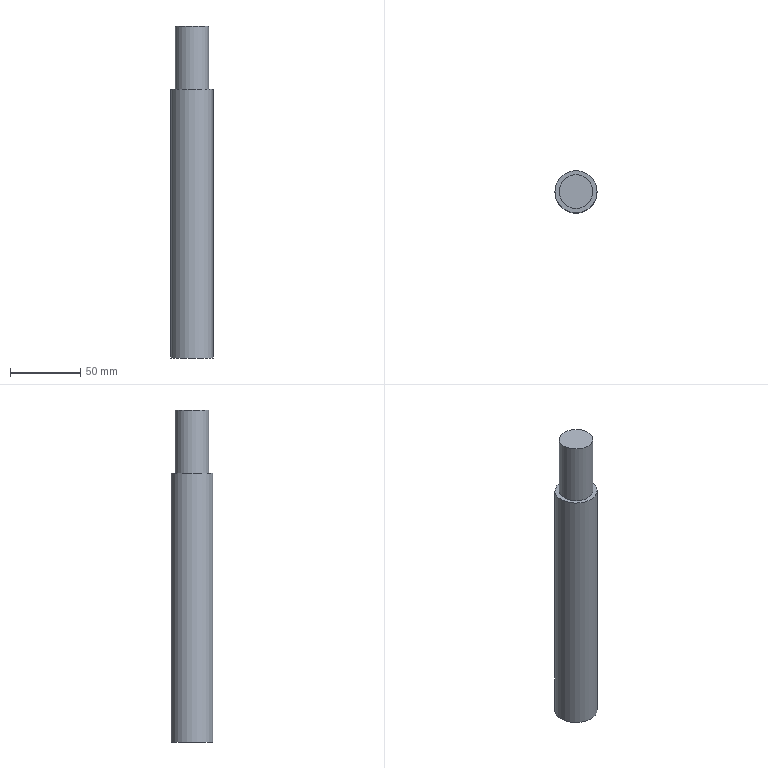Part | NX | features solid 2 | 1 solid | 5 faces | box 30 x 30 x 236 mm | volume 155367 mm3 | plane 3 | cylinder 2 | commonest cylinder face diameters 24 x1 30 x1
STEP:
#1=CARTESIAN_POINT('',(230.,77.5,-250.));
#2=VERTEX_POINT('',#1);
#3=CARTESIAN_POINT('',(215.,77.5,-250.));
#4=DIRECTION('',(0.,0.,1.));
#5=DIRECTION('',(1.,0.,0.));
#6=AXIS2_PLACEMENT_3D('',#3,#4,#5);
#7=CIRCLE('',#6,15.);
#8=EDGE_CURVE('',#2,#2,#7,.T.);
#9=ORIENTED_EDGE('',*,*,#8,.T.);
#10=EDGE_LOOP('',(#9));
#11=FACE_BOUND('',#10,.T.);
#12=CARTESIAN_POINT('',(230.,77.5,-59.));
#13=VERTEX_POINT('',#12);
#14=CARTESIAN_POINT('',(215.,77.5,-59.));
#15=DIRECTION('',(0.,0.,1.));
#16=DIRECTION('',(1.,0.,0.));
#17=AXIS2_PLACEMENT_3D('',#14,#15,#16);
#18=CIRCLE('',#17,15.);
#19=EDGE_CURVE('',#13,#13,#18,.T.);
#20=ORIENTED_EDGE('',*,*,#19,.F.);
#21=EDGE_LOOP('',(#20));
#22=FACE_BOUND('',#21,.T.);
#23=CARTESIAN_POINT('',(215.,77.5,-250.));
#24=DIRECTION('',(0.,0.,1.));
#25=DIRECTION('',(-1.,0.,0.));
#26=AXIS2_PLACEMENT_3D('',#23,#24,#25);
#27=CYLINDRICAL_SURFACE('',#26,15.);
#28=ADVANCED_FACE('',(#11,#22),#27,.T.);
#29=ORIENTED_EDGE('',*,*,#8,.F.);
#30=EDGE_LOOP('',(#29));
#31=FACE_BOUND('',#30,.T.);
#32=CARTESIAN_POINT('',(215.,77.5,-250.));
#33=DIRECTION('',(0.,0.,-1.));
#34=DIRECTION('',(1.,0.,0.));
#35=AXIS2_PLACEMENT_3D('',#32,#33,#34);
#36=PLANE('',#35);
#37=ADVANCED_FACE('',(#31),#36,.T.);
#38=CARTESIAN_POINT('',(227.,77.5,-59.));
#39=VERTEX_POINT('',#38);
#40=CARTESIAN_POINT('',(215.,77.5,-59.));
#41=DIRECTION('',(0.,0.,1.));
#42=DIRECTION('',(1.,0.,0.));
#43=AXIS2_PLACEMENT_3D('',#40,#41,#42);
#44=CIRCLE('',#43,12.);
#45=EDGE_CURVE('',#39,#39,#44,.T.);
#46=ORIENTED_EDGE('',*,*,#45,.F.);
#47=EDGE_LOOP('',(#46));
#48=FACE_BOUND('',#47,.T.);
#49=ORIENTED_EDGE('',*,*,#19,.T.);
#50=EDGE_LOOP('',(#49));
#51=FACE_BOUND('',#50,.T.);
#52=CARTESIAN_POINT('',(215.,77.5,-59.));
#53=DIRECTION('',(0.,0.,-1.));
#54=DIRECTION('',(1.,0.,0.));
#55=AXIS2_PLACEMENT_3D('',#52,#53,#54);
#56=PLANE('',#55);
#57=ADVANCED_FACE('',(#48,#51),#56,.F.);
#58=CARTESIAN_POINT('',(227.,77.5,-14.));
#59=VERTEX_POINT('',#58);
#60=CARTESIAN_POINT('',(215.,77.5,-14.));
#61=DIRECTION('',(0.,0.,1.));
#62=DIRECTION('',(1.,0.,0.));
#63=AXIS2_PLACEMENT_3D('',#60,#61,#62);
#64=CIRCLE('',#63,12.);
#65=EDGE_CURVE('',#59,#59,#64,.T.);
#66=ORIENTED_EDGE('',*,*,#65,.F.);
#67=EDGE_LOOP('',(#66));
#68=FACE_BOUND('',#67,.T.);
#69=ORIENTED_EDGE('',*,*,#45,.T.);
#70=EDGE_LOOP('',(#69));
#71=FACE_BOUND('',#70,.T.);
#72=CARTESIAN_POINT('',(215.,77.5,-10.));
#73=DIRECTION('',(0.,0.,-1.));
#74=DIRECTION('',(1.,0.,0.));
#75=AXIS2_PLACEMENT_3D('',#72,#73,#74);
#76=CYLINDRICAL_SURFACE('',#75,12.);
#77=ADVANCED_FACE('',(#68,#71),#76,.T.);
#78=ORIENTED_EDGE('',*,*,#65,.T.);
#79=EDGE_LOOP('',(#78));
#80=FACE_BOUND('',#79,.T.);
#81=CARTESIAN_POINT('',(215.,77.5,-14.));
#82=DIRECTION('',(0.,0.,-1.));
#83=DIRECTION('',(1.,0.,0.));
#84=AXIS2_PLACEMENT_3D('',#81,#82,#83);
#85=PLANE('',#84);
#86=ADVANCED_FACE('',(#80),#85,.F.);
#87=CLOSED_SHELL('',(#28,#37,#57,#77,#86));
#88=MANIFOLD_SOLID_BREP('',#87);
#89=(LENGTH_UNIT()NAMED_UNIT(*)SI_UNIT(.MILLI.,.METRE.));
#90=UNCERTAINTY_MEASURE_WITH_UNIT(LENGTH_MEASURE(0.00001),#89,'','');
#91=(NAMED_UNIT(*)PLANE_ANGLE_UNIT()SI_UNIT($,.RADIAN.));
#92=(NAMED_UNIT(*)SI_UNIT($,.STERADIAN.)SOLID_ANGLE_UNIT());
#93=(GEOMETRIC_REPRESENTATION_CONTEXT(3)GLOBAL_UNCERTAINTY_ASSIGNED_CONTEXT((#90))GLOBAL_UNIT_ASSIGNED_CONTEXT((#89,#91,#92))REPRESENTATION_CONTEXT('',''));
#94=ADVANCED_BREP_SHAPE_REPRESENTATION('',(#88),#93);